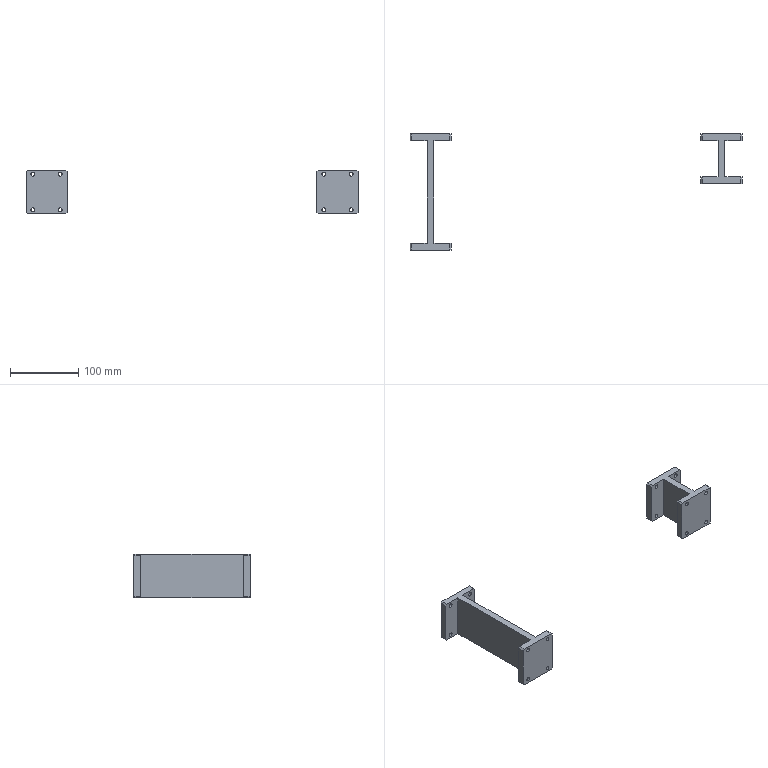Part | STEP file | Support plate | 2 solids | 76 faces | box 485 x 170 x 64 mm | volume 279239 mm3 | plane 44 | cylinder 32 | commonest cylinder face diameters 5.5 x32